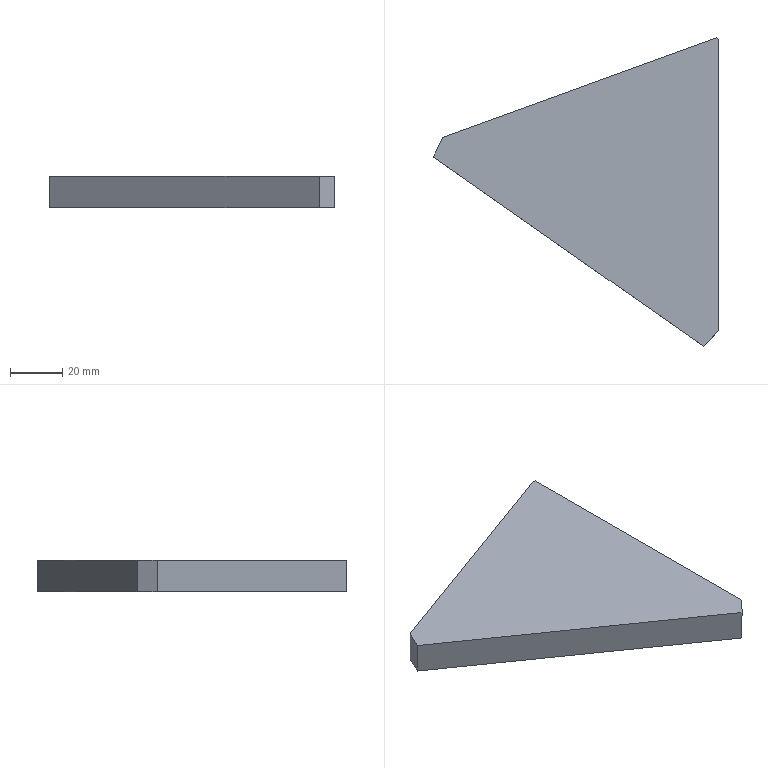Part | SolidWorks | features Chamfer 1, Extrusion 1 | 1 solid | 8 faces | box 109.653 x 118.533 x 12 mm | volume 84519 mm3 | plane 8
STEP:
#1=CARTESIAN_POINT('',(0.,242.859,-260.));
#2=VERTEX_POINT('',#1);
#3=CARTESIAN_POINT('',(-0.8192,243.433,-260.));
#4=VERTEX_POINT('',#3);
#5=CARTESIAN_POINT('',(-0.8192,243.433,-260.));
#6=DIRECTION('',(-0.8192,0.5736,0.));
#7=VECTOR('',#6,1000.);
#8=LINE('',#5,#7);
#9=EDGE_CURVE('',#2,#4,#8,.T.);
#10=ORIENTED_EDGE('',*,*,#9,.T.);
#11=CARTESIAN_POINT('',(-0.8192,243.433,-248.));
#12=VERTEX_POINT('',#11);
#13=CARTESIAN_POINT('',(-0.8192,243.433,-248.));
#14=DIRECTION('',(0.,0.,-1.));
#15=VECTOR('',#14,1000.);
#16=LINE('',#13,#15);
#17=EDGE_CURVE('',#12,#4,#16,.T.);
#18=ORIENTED_EDGE('',*,*,#17,.F.);
#19=CARTESIAN_POINT('',(0.,242.859,-248.));
#20=VERTEX_POINT('',#19);
#21=CARTESIAN_POINT('',(-0.8192,243.433,-248.));
#22=DIRECTION('',(-0.8192,0.5736,0.));
#23=VECTOR('',#22,1000.);
#24=LINE('',#21,#23);
#25=EDGE_CURVE('',#20,#12,#24,.T.);
#26=ORIENTED_EDGE('',*,*,#25,.F.);
#27=CARTESIAN_POINT('',(0.,242.859,-248.));
#28=DIRECTION('',(0.,0.,-1.));
#29=VECTOR('',#28,1000.);
#30=LINE('',#27,#29);
#31=EDGE_CURVE('',#20,#2,#30,.T.);
#32=ORIENTED_EDGE('',*,*,#31,.T.);
#33=EDGE_LOOP('',(#10,#18,#26,#32));
#34=FACE_OUTER_BOUND('',#33,.T.);
#35=CARTESIAN_POINT('',(-0.8192,243.433,-248.));
#36=DIRECTION('',(-0.5736,-0.8192,0.));
#37=DIRECTION('',(0.8192,-0.5736,0.));
#38=AXIS2_PLACEMENT_3D('',#35,#36,#37);
#39=PLANE('',#38);
#40=ADVANCED_FACE('',(#34),#39,.F.);
#41=CARTESIAN_POINT('',(-106.138,205.1,-260.));
#42=VERTEX_POINT('',#41);
#43=CARTESIAN_POINT('',(-0.8192,243.433,-260.));
#44=DIRECTION('',(-0.9397,-0.342,0.));
#45=VECTOR('',#44,1000.);
#46=LINE('',#43,#45);
#47=EDGE_CURVE('',#4,#42,#46,.T.);
#48=ORIENTED_EDGE('',*,*,#47,.T.);
#49=CARTESIAN_POINT('',(-106.138,205.1,-248.));
#50=VERTEX_POINT('',#49);
#51=CARTESIAN_POINT('',(-106.138,205.1,-248.));
#52=DIRECTION('',(0.,0.,1.));
#53=VECTOR('',#52,1000.);
#54=LINE('',#51,#53);
#55=EDGE_CURVE('',#42,#50,#54,.T.);
#56=ORIENTED_EDGE('',*,*,#55,.T.);
#57=CARTESIAN_POINT('',(-0.8192,243.433,-248.));
#58=DIRECTION('',(-0.9397,-0.342,0.));
#59=VECTOR('',#58,1000.);
#60=LINE('',#57,#59);
#61=EDGE_CURVE('',#12,#50,#60,.T.);
#62=ORIENTED_EDGE('',*,*,#61,.F.);
#63=ORIENTED_EDGE('',*,*,#17,.T.);
#64=EDGE_LOOP('',(#48,#56,#62,#63));
#65=FACE_OUTER_BOUND('',#64,.T.);
#66=CARTESIAN_POINT('',(-0.8192,243.433,-248.));
#67=DIRECTION('',(0.342,-0.9397,0.));
#68=DIRECTION('',(0.9397,0.342,0.));
#69=AXIS2_PLACEMENT_3D('',#66,#67,#68);
#70=PLANE('',#69);
#71=ADVANCED_FACE('',(#65),#70,.F.);
#72=CARTESIAN_POINT('',(-109.653,197.562,-260.));
#73=VERTEX_POINT('',#72);
#74=CARTESIAN_POINT('',(-5.882,124.9,-260.));
#75=VERTEX_POINT('',#74);
#76=CARTESIAN_POINT('',(-115.534,201.68,-260.));
#77=DIRECTION('',(0.8192,-0.5736,0.));
#78=VECTOR('',#77,1000.);
#79=LINE('',#76,#78);
#80=EDGE_CURVE('',#73,#75,#79,.T.);
#81=ORIENTED_EDGE('',*,*,#80,.T.);
#82=CARTESIAN_POINT('',(-5.882,124.9,-248.));
#83=VERTEX_POINT('',#82);
#84=CARTESIAN_POINT('',(-5.882,124.9,-248.));
#85=DIRECTION('',(0.,0.,1.));
#86=VECTOR('',#85,1000.);
#87=LINE('',#84,#86);
#88=EDGE_CURVE('',#75,#83,#87,.T.);
#89=ORIENTED_EDGE('',*,*,#88,.T.);
#90=CARTESIAN_POINT('',(-109.653,197.562,-248.));
#91=VERTEX_POINT('',#90);
#92=CARTESIAN_POINT('',(-115.534,201.68,-248.));
#93=DIRECTION('',(0.8192,-0.5736,0.));
#94=VECTOR('',#93,1000.);
#95=LINE('',#92,#94);
#96=EDGE_CURVE('',#91,#83,#95,.T.);
#97=ORIENTED_EDGE('',*,*,#96,.F.);
#98=CARTESIAN_POINT('',(-109.653,197.562,-248.));
#99=DIRECTION('',(0.,0.,-1.));
#100=VECTOR('',#99,1000.);
#101=LINE('',#98,#100);
#102=EDGE_CURVE('',#91,#73,#101,.T.);
#103=ORIENTED_EDGE('',*,*,#102,.T.);
#104=EDGE_LOOP('',(#81,#89,#97,#103));
#105=FACE_OUTER_BOUND('',#104,.T.);
#106=CARTESIAN_POINT('',(-115.534,201.68,-248.));
#107=DIRECTION('',(0.5736,0.8192,0.));
#108=DIRECTION('',(-0.8192,0.5736,0.));
#109=AXIS2_PLACEMENT_3D('',#106,#107,#108);
#110=PLANE('',#109);
#111=ADVANCED_FACE('',(#105),#110,.F.);
#112=CARTESIAN_POINT('',(0.,130.782,-248.));
#113=VERTEX_POINT('',#112);
#114=CARTESIAN_POINT('',(0.,120.782,-248.));
#115=DIRECTION('',(0.,1.,0.));
#116=VECTOR('',#115,1000.);
#117=LINE('',#114,#116);
#118=EDGE_CURVE('',#113,#20,#117,.T.);
#119=ORIENTED_EDGE('',*,*,#118,.F.);
#120=CARTESIAN_POINT('',(0.,130.782,-260.));
#121=VERTEX_POINT('',#120);
#122=CARTESIAN_POINT('',(0.,130.782,-248.));
#123=DIRECTION('',(0.,0.,-1.));
#124=VECTOR('',#123,1000.);
#125=LINE('',#122,#124);
#126=EDGE_CURVE('',#113,#121,#125,.T.);
#127=ORIENTED_EDGE('',*,*,#126,.T.);
#128=CARTESIAN_POINT('',(0.,120.782,-260.));
#129=DIRECTION('',(0.,1.,0.));
#130=VECTOR('',#129,1000.);
#131=LINE('',#128,#130);
#132=EDGE_CURVE('',#121,#2,#131,.T.);
#133=ORIENTED_EDGE('',*,*,#132,.T.);
#134=ORIENTED_EDGE('',*,*,#31,.F.);
#135=EDGE_LOOP('',(#119,#127,#133,#134));
#136=FACE_OUTER_BOUND('',#135,.T.);
#137=CARTESIAN_POINT('',(0.,120.782,-248.));
#138=DIRECTION('',(-1.,0.,0.));
#139=DIRECTION('',(0.,-1.,0.));
#140=AXIS2_PLACEMENT_3D('',#137,#138,#139);
#141=PLANE('',#140);
#142=ADVANCED_FACE('',(#136),#141,.F.);
#143=ORIENTED_EDGE('',*,*,#96,.T.);
#144=CARTESIAN_POINT('',(-65.391,65.391,-248.));
#145=DIRECTION('',(0.7071,0.7071,0.));
#146=VECTOR('',#145,1000.);
#147=LINE('',#144,#146);
#148=EDGE_CURVE('',#83,#113,#147,.T.);
#149=ORIENTED_EDGE('',*,*,#148,.T.);
#150=ORIENTED_EDGE('',*,*,#118,.T.);
#151=ORIENTED_EDGE('',*,*,#25,.T.);
#152=ORIENTED_EDGE('',*,*,#61,.T.);
#153=CARTESIAN_POINT('',(-165.739,77.285,-248.));
#154=DIRECTION('',(-0.4226,-0.9063,0.));
#155=VECTOR('',#154,1000.);
#156=LINE('',#153,#155);
#157=EDGE_CURVE('',#50,#91,#156,.T.);
#158=ORIENTED_EDGE('',*,*,#157,.T.);
#159=EDGE_LOOP('',(#143,#149,#150,#151,#152,#158));
#160=FACE_OUTER_BOUND('',#159,.T.);
#161=CARTESIAN_POINT('',(0.,0.,-248.));
#162=DIRECTION('',(0.,0.,1.));
#163=DIRECTION('',(1.,0.,0.));
#164=AXIS2_PLACEMENT_3D('',#161,#162,#163);
#165=PLANE('',#164);
#166=ADVANCED_FACE('',(#160),#165,.T.);
#167=ORIENTED_EDGE('',*,*,#132,.F.);
#168=CARTESIAN_POINT('',(0.,130.782,-260.));
#169=DIRECTION('',(-0.7071,-0.7071,0.));
#170=VECTOR('',#169,1000.);
#171=LINE('',#168,#170);
#172=EDGE_CURVE('',#121,#75,#171,.T.);
#173=ORIENTED_EDGE('',*,*,#172,.T.);
#174=ORIENTED_EDGE('',*,*,#80,.F.);
#175=CARTESIAN_POINT('',(-109.653,197.562,-260.));
#176=DIRECTION('',(0.4226,0.9063,0.));
#177=VECTOR('',#176,1000.);
#178=LINE('',#175,#177);
#179=EDGE_CURVE('',#73,#42,#178,.T.);
#180=ORIENTED_EDGE('',*,*,#179,.T.);
#181=ORIENTED_EDGE('',*,*,#47,.F.);
#182=ORIENTED_EDGE('',*,*,#9,.F.);
#183=EDGE_LOOP('',(#167,#173,#174,#180,#181,#182));
#184=FACE_OUTER_BOUND('',#183,.T.);
#185=CARTESIAN_POINT('',(0.,0.,-260.));
#186=DIRECTION('',(0.,0.,1.));
#187=DIRECTION('',(1.,0.,0.));
#188=AXIS2_PLACEMENT_3D('',#185,#186,#187);
#189=PLANE('',#188);
#190=ADVANCED_FACE('',(#184),#189,.F.);
#191=ORIENTED_EDGE('',*,*,#148,.F.);
#192=ORIENTED_EDGE('',*,*,#88,.F.);
#193=ORIENTED_EDGE('',*,*,#172,.F.);
#194=ORIENTED_EDGE('',*,*,#126,.F.);
#195=EDGE_LOOP('',(#191,#192,#193,#194));
#196=FACE_OUTER_BOUND('',#195,.T.);
#197=CARTESIAN_POINT('',(0.,130.782,-248.));
#198=DIRECTION('',(-0.7071,0.7071,0.));
#199=DIRECTION('',(0.,0.,-1.));
#200=AXIS2_PLACEMENT_3D('',#197,#198,#199);
#201=PLANE('',#200);
#202=ADVANCED_FACE('',(#196),#201,.F.);
#203=ORIENTED_EDGE('',*,*,#157,.F.);
#204=ORIENTED_EDGE('',*,*,#55,.F.);
#205=ORIENTED_EDGE('',*,*,#179,.F.);
#206=ORIENTED_EDGE('',*,*,#102,.F.);
#207=EDGE_LOOP('',(#203,#204,#205,#206));
#208=FACE_OUTER_BOUND('',#207,.T.);
#209=CARTESIAN_POINT('',(-109.653,197.562,-248.));
#210=DIRECTION('',(0.9063,-0.4226,0.));
#211=DIRECTION('',(0.,0.,-1.));
#212=AXIS2_PLACEMENT_3D('',#209,#210,#211);
#213=PLANE('',#212);
#214=ADVANCED_FACE('',(#208),#213,.F.);
#215=CLOSED_SHELL('',(#40,#71,#111,#142,#166,#190,#202,#214));
#216=MANIFOLD_SOLID_BREP('',#215);
#217=CARTESIAN_POINT('',(0.,0.,0.));
#218=DIRECTION('',(0.,0.,1.));
#219=DIRECTION('',(1.,0.,0.));
#220=AXIS2_PLACEMENT_3D('',#217,#218,#219);
#221=(LENGTH_UNIT()NAMED_UNIT(*)SI_UNIT(.MILLI.,.METRE.));
#222=UNCERTAINTY_MEASURE_WITH_UNIT(LENGTH_MEASURE(0.00001),#221,'','');
#223=(NAMED_UNIT(*)PLANE_ANGLE_UNIT()SI_UNIT($,.RADIAN.));
#224=(NAMED_UNIT(*)SI_UNIT($,.STERADIAN.)SOLID_ANGLE_UNIT());
#225=(GEOMETRIC_REPRESENTATION_CONTEXT(3)GLOBAL_UNCERTAINTY_ASSIGNED_CONTEXT((#222))GLOBAL_UNIT_ASSIGNED_CONTEXT((#221,#223,#224))REPRESENTATION_CONTEXT('',''));
#226=ADVANCED_BREP_SHAPE_REPRESENTATION('',(#216,#220),#225);